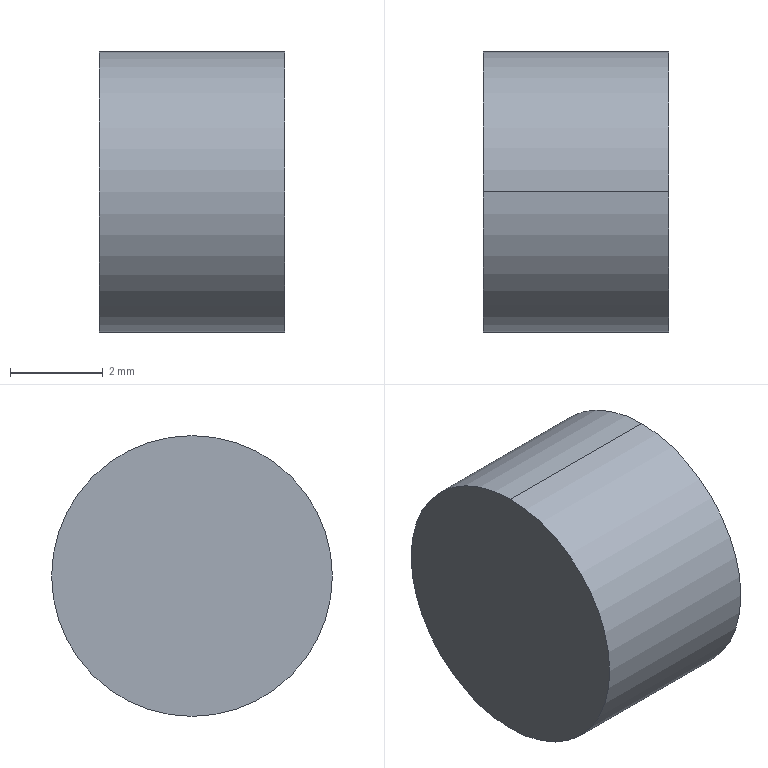Part | STEP file | _X2_7FC5724752A070ED7BA1_X0_1_4 | 1 solid | 4 faces | box 4 x 6.052 x 6.052 mm | volume 115.068 mm3 | cylinder 2 | plane 2 | commonest cylinder face diameters 6.052 x2
STEP:
#1=CARTESIAN_POINT('',(0.,0.,0.));
#2=DIRECTION('',(0.,0.,1.));
#3=DIRECTION('',(1.,0.,0.));
#4=AXIS2_PLACEMENT_3D('',#1,#2,#3);
#5=CARTESIAN_POINT('',(-41.,0.,3.026));
#6=VERTEX_POINT('',#5);
#7=CARTESIAN_POINT('',(-37.,0.,3.026));
#8=VERTEX_POINT('',#7);
#9=CARTESIAN_POINT('',(-41.,0.,3.026));
#10=DIRECTION('',(1.,0.,0.));
#11=VECTOR('',#10,1.);
#12=LINE('',#9,#11);
#13=CARTESIAN_POINT('',(-41.,0.,0.));
#14=DIRECTION('',(1.,0.,0.));
#15=DIRECTION('',(0.,0.,-1.));
#16=AXIS2_PLACEMENT_3D('',#13,#14,#15);
#17=CYLINDRICAL_SURFACE('',#16,3.026);
#18=CARTESIAN_POINT('',(3.142,0.));
#19=DIRECTION('',(0.,1.));
#20=VECTOR('',#19,1.);
#21=LINE('',#18,#20);
#22=(GEOMETRIC_REPRESENTATION_CONTEXT(2)PARAMETRIC_REPRESENTATION_CONTEXT()REPRESENTATION_CONTEXT('',''));
#23=DEFINITIONAL_REPRESENTATION('',(#21),#22);
#24=PCURVE('',#17,#23);
#25=CARTESIAN_POINT('',(-41.,0.,0.));
#26=DIRECTION('',(1.,0.,0.));
#27=DIRECTION('',(0.,0.,-1.));
#28=AXIS2_PLACEMENT_3D('',#25,#26,#27);
#29=CYLINDRICAL_SURFACE('',#28,3.026);
#30=CARTESIAN_POINT('',(3.142,0.));
#31=DIRECTION('',(0.,1.));
#32=VECTOR('',#31,1.);
#33=LINE('',#30,#32);
#34=(GEOMETRIC_REPRESENTATION_CONTEXT(2)PARAMETRIC_REPRESENTATION_CONTEXT()REPRESENTATION_CONTEXT('',''));
#35=DEFINITIONAL_REPRESENTATION('',(#33),#34);
#36=PCURVE('',#29,#35);
#37=SURFACE_CURVE('',#12,(#24,#36),.PCURVE_S1.);
#38=EDGE_CURVE('',#6,#8,#37,.T.);
#39=ORIENTED_EDGE('',*,*,#38,.T.);
#40=CARTESIAN_POINT('',(-37.,3.026,0.));
#41=VERTEX_POINT('',#40);
#42=CARTESIAN_POINT('',(-37.,0.,0.));
#43=DIRECTION('',(1.,0.,0.));
#44=DIRECTION('',(0.,1.,0.));
#45=AXIS2_PLACEMENT_3D('',#42,#43,#44);
#46=CIRCLE('',#45,3.026);
#47=CARTESIAN_POINT('',(1.571,4.));
#48=DIRECTION('',(1.,0.));
#49=VECTOR('',#48,1.);
#50=LINE('',#47,#49);
#51=(GEOMETRIC_REPRESENTATION_CONTEXT(2)PARAMETRIC_REPRESENTATION_CONTEXT()REPRESENTATION_CONTEXT('',''));
#52=DEFINITIONAL_REPRESENTATION('',(#50),#51);
#53=PCURVE('',#17,#52);
#54=CARTESIAN_POINT('',(-37.,0.,0.));
#55=DIRECTION('',(-1.,0.,0.));
#56=DIRECTION('',(0.,0.,1.));
#57=AXIS2_PLACEMENT_3D('',#54,#55,#56);
#58=PLANE('',#57);
#59=CARTESIAN_POINT('',(0.,3.026));
#60=CARTESIAN_POINT('',(5.241,3.026));
#61=CARTESIAN_POINT('',(2.621,-1.513));
#62=CARTESIAN_POINT('',(0.,-6.052));
#63=CARTESIAN_POINT('',(-2.621,-1.513));
#64=CARTESIAN_POINT('',(-5.241,3.026));
#65=CARTESIAN_POINT('',(0.,3.026));
#66=(BOUNDED_CURVE()B_SPLINE_CURVE(2,(#59,#60,#61,#62,#63,#64,#65),.UNSPECIFIED.,.T.,.F.)B_SPLINE_CURVE_WITH_KNOTS((1,2,2,2,2,1),(-2.094,0.,2.094,4.189,6.283,8.378),.UNSPECIFIED.)CURVE()GEOMETRIC_REPRESENTATION_ITEM()RATIONAL_B_SPLINE_CURVE((1.,0.5,1.,0.5,1.,0.5,1.))REPRESENTATION_ITEM(''));
#67=(GEOMETRIC_REPRESENTATION_CONTEXT(2)PARAMETRIC_REPRESENTATION_CONTEXT()REPRESENTATION_CONTEXT('',''));
#68=DEFINITIONAL_REPRESENTATION('',(#66),#67);
#69=PCURVE('',#58,#68);
#70=SURFACE_CURVE('',#46,(#53,#69),.PCURVE_S1.);
#71=EDGE_CURVE('',#41,#8,#70,.T.);
#72=ORIENTED_EDGE('',*,*,#71,.F.);
#73=CARTESIAN_POINT('',(-37.,0.,-3.026));
#74=VERTEX_POINT('',#73);
#75=CARTESIAN_POINT('',(-37.,0.,0.));
#76=DIRECTION('',(1.,0.,0.));
#77=DIRECTION('',(0.,0.,-1.));
#78=AXIS2_PLACEMENT_3D('',#75,#76,#77);
#79=CIRCLE('',#78,3.026);
#80=CARTESIAN_POINT('',(0.,4.));
#81=DIRECTION('',(1.,0.));
#82=VECTOR('',#81,1.);
#83=LINE('',#80,#82);
#84=(GEOMETRIC_REPRESENTATION_CONTEXT(2)PARAMETRIC_REPRESENTATION_CONTEXT()REPRESENTATION_CONTEXT('',''));
#85=DEFINITIONAL_REPRESENTATION('',(#83),#84);
#86=PCURVE('',#17,#85);
#87=CARTESIAN_POINT('',(-3.026,0.));
#88=CARTESIAN_POINT('',(-3.026,5.241));
#89=CARTESIAN_POINT('',(1.513,2.621));
#90=CARTESIAN_POINT('',(6.052,0.));
#91=CARTESIAN_POINT('',(1.513,-2.621));
#92=CARTESIAN_POINT('',(-3.026,-5.241));
#93=CARTESIAN_POINT('',(-3.026,0.));
#94=(BOUNDED_CURVE()B_SPLINE_CURVE(2,(#87,#88,#89,#90,#91,#92,#93),.UNSPECIFIED.,.T.,.F.)B_SPLINE_CURVE_WITH_KNOTS((1,2,2,2,2,1),(-2.094,0.,2.094,4.189,6.283,8.378),.UNSPECIFIED.)CURVE()GEOMETRIC_REPRESENTATION_ITEM()RATIONAL_B_SPLINE_CURVE((1.,0.5,1.,0.5,1.,0.5,1.))REPRESENTATION_ITEM(''));
#95=(GEOMETRIC_REPRESENTATION_CONTEXT(2)PARAMETRIC_REPRESENTATION_CONTEXT()REPRESENTATION_CONTEXT('',''));
#96=DEFINITIONAL_REPRESENTATION('',(#94),#95);
#97=PCURVE('',#58,#96);
#98=SURFACE_CURVE('',#79,(#86,#97),.PCURVE_S1.);
#99=EDGE_CURVE('',#74,#41,#98,.T.);
#100=ORIENTED_EDGE('',*,*,#99,.F.);
#101=CARTESIAN_POINT('',(-41.,0.,-3.026));
#102=VERTEX_POINT('',#101);
#103=CARTESIAN_POINT('',(-41.,0.,-3.026));
#104=DIRECTION('',(1.,0.,0.));
#105=VECTOR('',#104,1.);
#106=LINE('',#103,#105);
#107=CARTESIAN_POINT('',(0.,0.));
#108=DIRECTION('',(0.,1.));
#109=VECTOR('',#108,1.);
#110=LINE('',#107,#109);
#111=(GEOMETRIC_REPRESENTATION_CONTEXT(2)PARAMETRIC_REPRESENTATION_CONTEXT()REPRESENTATION_CONTEXT('',''));
#112=DEFINITIONAL_REPRESENTATION('',(#110),#111);
#113=PCURVE('',#17,#112);
#114=CARTESIAN_POINT('',(6.283,0.));
#115=DIRECTION('',(0.,1.));
#116=VECTOR('',#115,1.);
#117=LINE('',#114,#116);
#118=(GEOMETRIC_REPRESENTATION_CONTEXT(2)PARAMETRIC_REPRESENTATION_CONTEXT()REPRESENTATION_CONTEXT('',''));
#119=DEFINITIONAL_REPRESENTATION('',(#117),#118);
#120=PCURVE('',#29,#119);
#121=SURFACE_CURVE('',#106,(#113,#120),.PCURVE_S1.);
#122=EDGE_CURVE('',#102,#74,#121,.T.);
#123=ORIENTED_EDGE('',*,*,#122,.F.);
#124=CARTESIAN_POINT('',(-41.,3.026,0.));
#125=VERTEX_POINT('',#124);
#126=CARTESIAN_POINT('',(-41.,0.,0.));
#127=DIRECTION('',(-1.,0.,0.));
#128=DIRECTION('',(0.,1.,0.));
#129=AXIS2_PLACEMENT_3D('',#126,#127,#128);
#130=CIRCLE('',#129,3.026);
#131=CARTESIAN_POINT('',(1.571,0.));
#132=DIRECTION('',(-1.,0.));
#133=VECTOR('',#132,1.);
#134=LINE('',#131,#133);
#135=(GEOMETRIC_REPRESENTATION_CONTEXT(2)PARAMETRIC_REPRESENTATION_CONTEXT()REPRESENTATION_CONTEXT('',''));
#136=DEFINITIONAL_REPRESENTATION('',(#134),#135);
#137=PCURVE('',#17,#136);
#138=CARTESIAN_POINT('',(-41.,0.,0.));
#139=DIRECTION('',(-1.,0.,0.));
#140=DIRECTION('',(0.,0.,1.));
#141=AXIS2_PLACEMENT_3D('',#138,#139,#140);
#142=PLANE('',#141);
#143=CARTESIAN_POINT('',(0.,0.));
#144=DIRECTION('',(0.,1.));
#145=AXIS2_PLACEMENT_2D('',#143,#144);
#146=CIRCLE('',#145,3.026);
#147=(GEOMETRIC_REPRESENTATION_CONTEXT(2)PARAMETRIC_REPRESENTATION_CONTEXT()REPRESENTATION_CONTEXT('',''));
#148=DEFINITIONAL_REPRESENTATION('',(#146),#147);
#149=PCURVE('',#142,#148);
#150=SURFACE_CURVE('',#130,(#137,#149),.PCURVE_S1.);
#151=EDGE_CURVE('',#125,#102,#150,.T.);
#152=ORIENTED_EDGE('',*,*,#151,.F.);
#153=CARTESIAN_POINT('',(-41.,0.,0.));
#154=DIRECTION('',(-1.,0.,0.));
#155=DIRECTION('',(0.,0.,1.));
#156=AXIS2_PLACEMENT_3D('',#153,#154,#155);
#157=CIRCLE('',#156,3.026);
#158=CARTESIAN_POINT('',(3.142,0.));
#159=DIRECTION('',(-1.,0.));
#160=VECTOR('',#159,1.);
#161=LINE('',#158,#160);
#162=(GEOMETRIC_REPRESENTATION_CONTEXT(2)PARAMETRIC_REPRESENTATION_CONTEXT()REPRESENTATION_CONTEXT('',''));
#163=DEFINITIONAL_REPRESENTATION('',(#161),#162);
#164=PCURVE('',#17,#163);
#165=CARTESIAN_POINT('',(0.,0.));
#166=DIRECTION('',(1.,0.));
#167=AXIS2_PLACEMENT_2D('',#165,#166);
#168=CIRCLE('',#167,3.026);
#169=(GEOMETRIC_REPRESENTATION_CONTEXT(2)PARAMETRIC_REPRESENTATION_CONTEXT()REPRESENTATION_CONTEXT('',''));
#170=DEFINITIONAL_REPRESENTATION('',(#168),#169);
#171=PCURVE('',#142,#170);
#172=SURFACE_CURVE('',#157,(#164,#171),.PCURVE_S1.);
#173=EDGE_CURVE('',#6,#125,#172,.T.);
#174=ORIENTED_EDGE('',*,*,#173,.F.);
#175=EDGE_LOOP('',(#39,#72,#100,#123,#152,#174));
#176=FACE_BOUND('',#175,.T.);
#177=ADVANCED_FACE('',(#176),#17,.T.);
#178=ORIENTED_EDGE('',*,*,#151,.F.);
#179=ORIENTED_EDGE('',*,*,#173,.F.);
#180=CARTESIAN_POINT('',(-41.,-3.026,0.));
#181=VERTEX_POINT('',#180);
#182=CARTESIAN_POINT('',(-41.,0.,0.));
#183=DIRECTION('',(-1.,0.,0.));
#184=DIRECTION('',(0.,-1.,0.));
#185=AXIS2_PLACEMENT_3D('',#182,#183,#184);
#186=CIRCLE('',#185,3.026);
#187=CARTESIAN_POINT('',(0.,0.));
#188=DIRECTION('',(0.,-1.));
#189=AXIS2_PLACEMENT_2D('',#187,#188);
#190=CIRCLE('',#189,3.026);
#191=(GEOMETRIC_REPRESENTATION_CONTEXT(2)PARAMETRIC_REPRESENTATION_CONTEXT()REPRESENTATION_CONTEXT('',''));
#192=DEFINITIONAL_REPRESENTATION('',(#190),#191);
#193=PCURVE('',#142,#192);
#194=CARTESIAN_POINT('',(4.712,0.));
#195=DIRECTION('',(-1.,0.));
#196=VECTOR('',#195,1.);
#197=LINE('',#194,#196);
#198=(GEOMETRIC_REPRESENTATION_CONTEXT(2)PARAMETRIC_REPRESENTATION_CONTEXT()REPRESENTATION_CONTEXT('',''));
#199=DEFINITIONAL_REPRESENTATION('',(#197),#198);
#200=PCURVE('',#29,#199);
#201=SURFACE_CURVE('',#186,(#193,#200),.PCURVE_S1.);
#202=EDGE_CURVE('',#181,#6,#201,.T.);
#203=ORIENTED_EDGE('',*,*,#202,.F.);
#204=CARTESIAN_POINT('',(-41.,0.,0.));
#205=DIRECTION('',(-1.,0.,0.));
#206=DIRECTION('',(0.,0.,-1.));
#207=AXIS2_PLACEMENT_3D('',#204,#205,#206);
#208=CIRCLE('',#207,3.026);
#209=CARTESIAN_POINT('',(0.,0.));
#210=DIRECTION('',(-1.,0.));
#211=AXIS2_PLACEMENT_2D('',#209,#210);
#212=CIRCLE('',#211,3.026);
#213=(GEOMETRIC_REPRESENTATION_CONTEXT(2)PARAMETRIC_REPRESENTATION_CONTEXT()REPRESENTATION_CONTEXT('',''));
#214=DEFINITIONAL_REPRESENTATION('',(#212),#213);
#215=PCURVE('',#142,#214);
#216=CARTESIAN_POINT('',(6.283,0.));
#217=DIRECTION('',(-1.,0.));
#218=VECTOR('',#217,1.);
#219=LINE('',#216,#218);
#220=(GEOMETRIC_REPRESENTATION_CONTEXT(2)PARAMETRIC_REPRESENTATION_CONTEXT()REPRESENTATION_CONTEXT('',''));
#221=DEFINITIONAL_REPRESENTATION('',(#219),#220);
#222=PCURVE('',#29,#221);
#223=SURFACE_CURVE('',#208,(#215,#222),.PCURVE_S1.);
#224=EDGE_CURVE('',#102,#181,#223,.T.);
#225=ORIENTED_EDGE('',*,*,#224,.F.);
#226=EDGE_LOOP('',(#178,#179,#203,#225));
#227=FACE_BOUND('',#226,.F.);
#228=ADVANCED_FACE('',(#227),#142,.T.);
#229=ORIENTED_EDGE('',*,*,#224,.F.);
#230=ORIENTED_EDGE('',*,*,#122,.T.);
#231=CARTESIAN_POINT('',(-37.,0.,0.));
#232=DIRECTION('',(1.,0.,0.));
#233=DIRECTION('',(0.,0.,1.));
#234=AXIS2_PLACEMENT_3D('',#231,#232,#233);
#235=CIRCLE('',#234,3.026);
#236=CARTESIAN_POINT('',(3.142,4.));
#237=DIRECTION('',(1.,0.));
#238=VECTOR('',#237,1.);
#239=LINE('',#236,#238);
#240=(GEOMETRIC_REPRESENTATION_CONTEXT(2)PARAMETRIC_REPRESENTATION_CONTEXT()REPRESENTATION_CONTEXT('',''));
#241=DEFINITIONAL_REPRESENTATION('',(#239),#240);
#242=PCURVE('',#29,#241);
#243=CARTESIAN_POINT('',(3.026,0.));
#244=CARTESIAN_POINT('',(3.026,-5.241));
#245=CARTESIAN_POINT('',(-1.513,-2.621));
#246=CARTESIAN_POINT('',(-6.052,0.));
#247=CARTESIAN_POINT('',(-1.513,2.621));
#248=CARTESIAN_POINT('',(3.026,5.241));
#249=CARTESIAN_POINT('',(3.026,0.));
#250=(BOUNDED_CURVE()B_SPLINE_CURVE(2,(#243,#244,#245,#246,#247,#248,#249),.UNSPECIFIED.,.T.,.F.)B_SPLINE_CURVE_WITH_KNOTS((1,2,2,2,2,1),(-2.094,0.,2.094,4.189,6.283,8.378),.UNSPECIFIED.)CURVE()GEOMETRIC_REPRESENTATION_ITEM()RATIONAL_B_SPLINE_CURVE((1.,0.5,1.,0.5,1.,0.5,1.))REPRESENTATION_ITEM(''));
#251=(GEOMETRIC_REPRESENTATION_CONTEXT(2)PARAMETRIC_REPRESENTATION_CONTEXT()REPRESENTATION_CONTEXT('',''));
#252=DEFINITIONAL_REPRESENTATION('',(#250),#251);
#253=PCURVE('',#58,#252);
#254=SURFACE_CURVE('',#235,(#242,#253),.PCURVE_S1.);
#255=EDGE_CURVE('',#8,#74,#254,.T.);
#256=ORIENTED_EDGE('',*,*,#255,.F.);
#257=ORIENTED_EDGE('',*,*,#38,.F.);
#258=ORIENTED_EDGE('',*,*,#202,.F.);
#259=EDGE_LOOP('',(#229,#230,#256,#257,#258));
#260=FACE_BOUND('',#259,.T.);
#261=ADVANCED_FACE('',(#260),#29,.T.);
#262=ORIENTED_EDGE('',*,*,#71,.F.);
#263=ORIENTED_EDGE('',*,*,#99,.F.);
#264=ORIENTED_EDGE('',*,*,#255,.F.);
#265=EDGE_LOOP('',(#262,#263,#264));
#266=FACE_BOUND('',#265,.F.);
#267=ADVANCED_FACE('',(#266),#58,.F.);
#268=CLOSED_SHELL('',(#177,#228,#261,#267));
#269=MANIFOLD_SOLID_BREP('',#268);
#270=(LENGTH_UNIT()NAMED_UNIT(*)SI_UNIT(.MILLI.,.METRE.));
#271=UNCERTAINTY_MEASURE_WITH_UNIT(LENGTH_MEASURE(0.0000001),#270,'','');
#272=(NAMED_UNIT(*)PLANE_ANGLE_UNIT()SI_UNIT($,.RADIAN.));
#273=(NAMED_UNIT(*)SI_UNIT($,.STERADIAN.)SOLID_ANGLE_UNIT());
#274=(GEOMETRIC_REPRESENTATION_CONTEXT(3)GLOBAL_UNCERTAINTY_ASSIGNED_CONTEXT((#271))GLOBAL_UNIT_ASSIGNED_CONTEXT((#270,#272,#273))REPRESENTATION_CONTEXT('',''));
#275=ADVANCED_BREP_SHAPE_REPRESENTATION('',(#4,#269),#274);